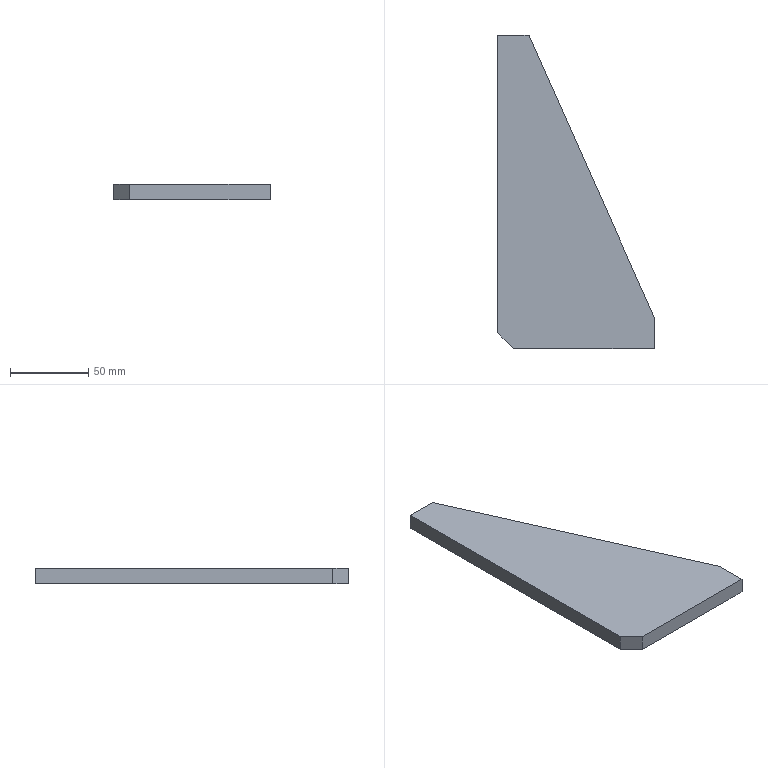Part | STEP file | Column base rib plate 1 | 1 solid | 8 faces | box 100 x 200 x 10 mm | volume 127500 mm3 | plane 8
STEP:
#1=CARTESIAN_POINT('',(0.,0.,0.));
#2=DIRECTION('',(0.,0.,1.));
#3=DIRECTION('',(1.,0.,0.));
#4=AXIS2_PLACEMENT_3D('',#1,#2,#3);
#5=CARTESIAN_POINT('',(0.,200.,-5.));
#6=VERTEX_POINT('',#5);
#7=CARTESIAN_POINT('',(0.,10.,-5.));
#8=VERTEX_POINT('',#7);
#9=CARTESIAN_POINT('',(0.,0.,-5.));
#10=DIRECTION('',(0.,-1.,0.));
#11=VECTOR('',#10,1.);
#12=LINE('',#9,#11);
#13=CARTESIAN_POINT('',(0.,0.,5.));
#14=DIRECTION('',(1.,0.,0.));
#15=DIRECTION('',(0.,0.,-1.));
#16=AXIS2_PLACEMENT_3D('',#13,#14,#15);
#17=PLANE('',#16);
#18=CARTESIAN_POINT('',(10.,0.));
#19=DIRECTION('',(0.,-1.));
#20=VECTOR('',#19,1.);
#21=LINE('',#18,#20);
#22=(GEOMETRIC_REPRESENTATION_CONTEXT(2)PARAMETRIC_REPRESENTATION_CONTEXT()REPRESENTATION_CONTEXT('',''));
#23=DEFINITIONAL_REPRESENTATION('',(#21),#22);
#24=PCURVE('',#17,#23);
#25=CARTESIAN_POINT('',(0.,0.,-5.));
#26=DIRECTION('',(0.,0.,-1.));
#27=DIRECTION('',(-1.,0.,0.));
#28=AXIS2_PLACEMENT_3D('',#25,#26,#27);
#29=PLANE('',#28);
#30=CARTESIAN_POINT('',(0.,0.));
#31=DIRECTION('',(0.,-1.));
#32=VECTOR('',#31,1.);
#33=LINE('',#30,#32);
#34=(GEOMETRIC_REPRESENTATION_CONTEXT(2)PARAMETRIC_REPRESENTATION_CONTEXT()REPRESENTATION_CONTEXT('',''));
#35=DEFINITIONAL_REPRESENTATION('',(#33),#34);
#36=PCURVE('',#29,#35);
#37=SURFACE_CURVE('',#12,(#24,#36),.PCURVE_S1.);
#38=EDGE_CURVE('',#6,#8,#37,.T.);
#39=ORIENTED_EDGE('',*,*,#38,.T.);
#40=CARTESIAN_POINT('',(0.,10.,5.));
#41=VERTEX_POINT('',#40);
#42=CARTESIAN_POINT('',(0.,10.,5.));
#43=DIRECTION('',(0.,0.,1.));
#44=VECTOR('',#43,1.);
#45=LINE('',#42,#44);
#46=CARTESIAN_POINT('',(0.,10.));
#47=DIRECTION('',(-1.,0.));
#48=VECTOR('',#47,1.);
#49=LINE('',#46,#48);
#50=(GEOMETRIC_REPRESENTATION_CONTEXT(2)PARAMETRIC_REPRESENTATION_CONTEXT()REPRESENTATION_CONTEXT('',''));
#51=DEFINITIONAL_REPRESENTATION('',(#49),#50);
#52=PCURVE('',#17,#51);
#53=CARTESIAN_POINT('',(10.,0.,5.));
#54=DIRECTION('',(0.7071,0.7071,0.));
#55=DIRECTION('',(0.,0.,-1.));
#56=AXIS2_PLACEMENT_3D('',#53,#54,#55);
#57=PLANE('',#56);
#58=CARTESIAN_POINT('',(0.,14.142));
#59=DIRECTION('',(-1.,0.));
#60=VECTOR('',#59,1.);
#61=LINE('',#58,#60);
#62=(GEOMETRIC_REPRESENTATION_CONTEXT(2)PARAMETRIC_REPRESENTATION_CONTEXT()REPRESENTATION_CONTEXT('',''));
#63=DEFINITIONAL_REPRESENTATION('',(#61),#62);
#64=PCURVE('',#57,#63);
#65=SURFACE_CURVE('',#45,(#52,#64),.PCURVE_S1.);
#66=EDGE_CURVE('',#8,#41,#65,.T.);
#67=ORIENTED_EDGE('',*,*,#66,.T.);
#68=CARTESIAN_POINT('',(0.,200.,5.));
#69=VERTEX_POINT('',#68);
#70=CARTESIAN_POINT('',(0.,0.,5.));
#71=DIRECTION('',(0.,-1.,0.));
#72=VECTOR('',#71,1.);
#73=LINE('',#70,#72);
#74=CARTESIAN_POINT('',(0.,0.));
#75=DIRECTION('',(0.,-1.));
#76=VECTOR('',#75,1.);
#77=LINE('',#74,#76);
#78=(GEOMETRIC_REPRESENTATION_CONTEXT(2)PARAMETRIC_REPRESENTATION_CONTEXT()REPRESENTATION_CONTEXT('',''));
#79=DEFINITIONAL_REPRESENTATION('',(#77),#78);
#80=PCURVE('',#17,#79);
#81=CARTESIAN_POINT('',(0.,0.,5.));
#82=DIRECTION('',(0.,0.,-1.));
#83=DIRECTION('',(-1.,0.,0.));
#84=AXIS2_PLACEMENT_3D('',#81,#82,#83);
#85=PLANE('',#84);
#86=CARTESIAN_POINT('',(0.,0.));
#87=DIRECTION('',(0.,-1.));
#88=VECTOR('',#87,1.);
#89=LINE('',#86,#88);
#90=(GEOMETRIC_REPRESENTATION_CONTEXT(2)PARAMETRIC_REPRESENTATION_CONTEXT()REPRESENTATION_CONTEXT('',''));
#91=DEFINITIONAL_REPRESENTATION('',(#89),#90);
#92=PCURVE('',#85,#91);
#93=SURFACE_CURVE('',#73,(#80,#92),.PCURVE_S1.);
#94=EDGE_CURVE('',#69,#41,#93,.T.);
#95=ORIENTED_EDGE('',*,*,#94,.F.);
#96=CARTESIAN_POINT('',(0.,200.,5.));
#97=DIRECTION('',(0.,0.,-1.));
#98=VECTOR('',#97,1.);
#99=LINE('',#96,#98);
#100=CARTESIAN_POINT('',(0.,200.));
#101=DIRECTION('',(1.,0.));
#102=VECTOR('',#101,1.);
#103=LINE('',#100,#102);
#104=(GEOMETRIC_REPRESENTATION_CONTEXT(2)PARAMETRIC_REPRESENTATION_CONTEXT()REPRESENTATION_CONTEXT('',''));
#105=DEFINITIONAL_REPRESENTATION('',(#103),#104);
#106=PCURVE('',#17,#105);
#107=CARTESIAN_POINT('',(0.,200.,5.));
#108=DIRECTION('',(0.,-1.,0.));
#109=DIRECTION('',(0.,0.,-1.));
#110=AXIS2_PLACEMENT_3D('',#107,#108,#109);
#111=PLANE('',#110);
#112=CARTESIAN_POINT('',(0.,0.));
#113=DIRECTION('',(1.,0.));
#114=VECTOR('',#113,1.);
#115=LINE('',#112,#114);
#116=(GEOMETRIC_REPRESENTATION_CONTEXT(2)PARAMETRIC_REPRESENTATION_CONTEXT()REPRESENTATION_CONTEXT('',''));
#117=DEFINITIONAL_REPRESENTATION('',(#115),#116);
#118=PCURVE('',#111,#117);
#119=SURFACE_CURVE('',#99,(#106,#118),.PCURVE_S1.);
#120=EDGE_CURVE('',#69,#6,#119,.T.);
#121=ORIENTED_EDGE('',*,*,#120,.T.);
#122=EDGE_LOOP('',(#39,#67,#95,#121));
#123=FACE_BOUND('',#122,.T.);
#124=ADVANCED_FACE('',(#123),#17,.F.);
#125=CARTESIAN_POINT('',(10.,0.,5.));
#126=VERTEX_POINT('',#125);
#127=CARTESIAN_POINT('',(100.,0.,5.));
#128=VERTEX_POINT('',#127);
#129=CARTESIAN_POINT('',(0.,0.,5.));
#130=DIRECTION('',(1.,0.,0.));
#131=VECTOR('',#130,1.);
#132=LINE('',#129,#131);
#133=CARTESIAN_POINT('',(0.,0.,5.));
#134=DIRECTION('',(0.,1.,0.));
#135=DIRECTION('',(0.,0.,1.));
#136=AXIS2_PLACEMENT_3D('',#133,#134,#135);
#137=PLANE('',#136);
#138=CARTESIAN_POINT('',(0.,0.));
#139=DIRECTION('',(0.,1.));
#140=VECTOR('',#139,1.);
#141=LINE('',#138,#140);
#142=(GEOMETRIC_REPRESENTATION_CONTEXT(2)PARAMETRIC_REPRESENTATION_CONTEXT()REPRESENTATION_CONTEXT('',''));
#143=DEFINITIONAL_REPRESENTATION('',(#141),#142);
#144=PCURVE('',#137,#143);
#145=CARTESIAN_POINT('',(0.,0.));
#146=DIRECTION('',(-1.,0.));
#147=VECTOR('',#146,1.);
#148=LINE('',#145,#147);
#149=(GEOMETRIC_REPRESENTATION_CONTEXT(2)PARAMETRIC_REPRESENTATION_CONTEXT()REPRESENTATION_CONTEXT('',''));
#150=DEFINITIONAL_REPRESENTATION('',(#148),#149);
#151=PCURVE('',#85,#150);
#152=SURFACE_CURVE('',#132,(#144,#151),.PCURVE_S1.);
#153=EDGE_CURVE('',#126,#128,#152,.T.);
#154=ORIENTED_EDGE('',*,*,#153,.F.);
#155=CARTESIAN_POINT('',(10.,0.,-5.));
#156=VERTEX_POINT('',#155);
#157=CARTESIAN_POINT('',(10.,0.,5.));
#158=DIRECTION('',(0.,0.,-1.));
#159=VECTOR('',#158,1.);
#160=LINE('',#157,#159);
#161=CARTESIAN_POINT('',(0.,10.));
#162=DIRECTION('',(-1.,0.));
#163=VECTOR('',#162,1.);
#164=LINE('',#161,#163);
#165=(GEOMETRIC_REPRESENTATION_CONTEXT(2)PARAMETRIC_REPRESENTATION_CONTEXT()REPRESENTATION_CONTEXT('',''));
#166=DEFINITIONAL_REPRESENTATION('',(#164),#165);
#167=PCURVE('',#137,#166);
#168=CARTESIAN_POINT('',(0.,0.));
#169=DIRECTION('',(1.,0.));
#170=VECTOR('',#169,1.);
#171=LINE('',#168,#170);
#172=(GEOMETRIC_REPRESENTATION_CONTEXT(2)PARAMETRIC_REPRESENTATION_CONTEXT()REPRESENTATION_CONTEXT('',''));
#173=DEFINITIONAL_REPRESENTATION('',(#171),#172);
#174=PCURVE('',#57,#173);
#175=SURFACE_CURVE('',#160,(#167,#174),.PCURVE_S1.);
#176=EDGE_CURVE('',#126,#156,#175,.T.);
#177=ORIENTED_EDGE('',*,*,#176,.T.);
#178=CARTESIAN_POINT('',(100.,0.,-5.));
#179=VERTEX_POINT('',#178);
#180=CARTESIAN_POINT('',(0.,0.,-5.));
#181=DIRECTION('',(1.,0.,0.));
#182=VECTOR('',#181,1.);
#183=LINE('',#180,#182);
#184=CARTESIAN_POINT('',(-10.,0.));
#185=DIRECTION('',(0.,1.));
#186=VECTOR('',#185,1.);
#187=LINE('',#184,#186);
#188=(GEOMETRIC_REPRESENTATION_CONTEXT(2)PARAMETRIC_REPRESENTATION_CONTEXT()REPRESENTATION_CONTEXT('',''));
#189=DEFINITIONAL_REPRESENTATION('',(#187),#188);
#190=PCURVE('',#137,#189);
#191=CARTESIAN_POINT('',(0.,0.));
#192=DIRECTION('',(-1.,0.));
#193=VECTOR('',#192,1.);
#194=LINE('',#191,#193);
#195=(GEOMETRIC_REPRESENTATION_CONTEXT(2)PARAMETRIC_REPRESENTATION_CONTEXT()REPRESENTATION_CONTEXT('',''));
#196=DEFINITIONAL_REPRESENTATION('',(#194),#195);
#197=PCURVE('',#29,#196);
#198=SURFACE_CURVE('',#183,(#190,#197),.PCURVE_S1.);
#199=EDGE_CURVE('',#156,#179,#198,.T.);
#200=ORIENTED_EDGE('',*,*,#199,.T.);
#201=CARTESIAN_POINT('',(100.,0.,5.));
#202=DIRECTION('',(0.,0.,-1.));
#203=VECTOR('',#202,1.);
#204=LINE('',#201,#203);
#205=CARTESIAN_POINT('',(0.,100.));
#206=DIRECTION('',(-1.,0.));
#207=VECTOR('',#206,1.);
#208=LINE('',#205,#207);
#209=(GEOMETRIC_REPRESENTATION_CONTEXT(2)PARAMETRIC_REPRESENTATION_CONTEXT()REPRESENTATION_CONTEXT('',''));
#210=DEFINITIONAL_REPRESENTATION('',(#208),#209);
#211=PCURVE('',#137,#210);
#212=CARTESIAN_POINT('',(100.,0.,5.));
#213=DIRECTION('',(-1.,0.,0.));
#214=DIRECTION('',(0.,-1.,0.));
#215=AXIS2_PLACEMENT_3D('',#212,#213,#214);
#216=PLANE('',#215);
#217=CARTESIAN_POINT('',(0.,0.));
#218=DIRECTION('',(0.,-1.));
#219=VECTOR('',#218,1.);
#220=LINE('',#217,#219);
#221=(GEOMETRIC_REPRESENTATION_CONTEXT(2)PARAMETRIC_REPRESENTATION_CONTEXT()REPRESENTATION_CONTEXT('',''));
#222=DEFINITIONAL_REPRESENTATION('',(#220),#221);
#223=PCURVE('',#216,#222);
#224=SURFACE_CURVE('',#204,(#211,#223),.PCURVE_S1.);
#225=EDGE_CURVE('',#128,#179,#224,.T.);
#226=ORIENTED_EDGE('',*,*,#225,.F.);
#227=EDGE_LOOP('',(#154,#177,#200,#226));
#228=FACE_BOUND('',#227,.T.);
#229=ADVANCED_FACE('',(#228),#137,.F.);
#230=CARTESIAN_POINT('',(100.,20.,-5.));
#231=VERTEX_POINT('',#230);
#232=CARTESIAN_POINT('',(100.,0.,-5.));
#233=DIRECTION('',(0.,1.,0.));
#234=VECTOR('',#233,1.);
#235=LINE('',#232,#234);
#236=CARTESIAN_POINT('',(0.,-10.));
#237=DIRECTION('',(-1.,0.));
#238=VECTOR('',#237,1.);
#239=LINE('',#236,#238);
#240=(GEOMETRIC_REPRESENTATION_CONTEXT(2)PARAMETRIC_REPRESENTATION_CONTEXT()REPRESENTATION_CONTEXT('',''));
#241=DEFINITIONAL_REPRESENTATION('',(#239),#240);
#242=PCURVE('',#216,#241);
#243=CARTESIAN_POINT('',(-100.,0.));
#244=DIRECTION('',(0.,1.));
#245=VECTOR('',#244,1.);
#246=LINE('',#243,#245);
#247=(GEOMETRIC_REPRESENTATION_CONTEXT(2)PARAMETRIC_REPRESENTATION_CONTEXT()REPRESENTATION_CONTEXT('',''));
#248=DEFINITIONAL_REPRESENTATION('',(#246),#247);
#249=PCURVE('',#29,#248);
#250=SURFACE_CURVE('',#235,(#242,#249),.PCURVE_S1.);
#251=EDGE_CURVE('',#179,#231,#250,.T.);
#252=ORIENTED_EDGE('',*,*,#251,.T.);
#253=CARTESIAN_POINT('',(100.,20.,5.));
#254=VERTEX_POINT('',#253);
#255=CARTESIAN_POINT('',(100.,20.,5.));
#256=DIRECTION('',(0.,0.,-1.));
#257=VECTOR('',#256,1.);
#258=LINE('',#255,#257);
#259=CARTESIAN_POINT('',(-20.,0.));
#260=DIRECTION('',(0.,-1.));
#261=VECTOR('',#260,1.);
#262=LINE('',#259,#261);
#263=(GEOMETRIC_REPRESENTATION_CONTEXT(2)PARAMETRIC_REPRESENTATION_CONTEXT()REPRESENTATION_CONTEXT('',''));
#264=DEFINITIONAL_REPRESENTATION('',(#262),#263);
#265=PCURVE('',#216,#264);
#266=CARTESIAN_POINT('',(100.,20.,5.));
#267=DIRECTION('',(-0.9138,-0.4061,0.));
#268=DIRECTION('',(0.4061,-0.9138,0.));
#269=AXIS2_PLACEMENT_3D('',#266,#267,#268);
#270=PLANE('',#269);
#271=CARTESIAN_POINT('',(0.,0.));
#272=DIRECTION('',(0.,-1.));
#273=VECTOR('',#272,1.);
#274=LINE('',#271,#273);
#275=(GEOMETRIC_REPRESENTATION_CONTEXT(2)PARAMETRIC_REPRESENTATION_CONTEXT()REPRESENTATION_CONTEXT('',''));
#276=DEFINITIONAL_REPRESENTATION('',(#274),#275);
#277=PCURVE('',#270,#276);
#278=SURFACE_CURVE('',#258,(#265,#277),.PCURVE_S1.);
#279=EDGE_CURVE('',#254,#231,#278,.T.);
#280=ORIENTED_EDGE('',*,*,#279,.F.);
#281=CARTESIAN_POINT('',(100.,0.,5.));
#282=DIRECTION('',(0.,1.,0.));
#283=VECTOR('',#282,1.);
#284=LINE('',#281,#283);
#285=CARTESIAN_POINT('',(0.,0.));
#286=DIRECTION('',(-1.,0.));
#287=VECTOR('',#286,1.);
#288=LINE('',#285,#287);
#289=(GEOMETRIC_REPRESENTATION_CONTEXT(2)PARAMETRIC_REPRESENTATION_CONTEXT()REPRESENTATION_CONTEXT('',''));
#290=DEFINITIONAL_REPRESENTATION('',(#288),#289);
#291=PCURVE('',#216,#290);
#292=CARTESIAN_POINT('',(-100.,0.));
#293=DIRECTION('',(0.,1.));
#294=VECTOR('',#293,1.);
#295=LINE('',#292,#294);
#296=(GEOMETRIC_REPRESENTATION_CONTEXT(2)PARAMETRIC_REPRESENTATION_CONTEXT()REPRESENTATION_CONTEXT('',''));
#297=DEFINITIONAL_REPRESENTATION('',(#295),#296);
#298=PCURVE('',#85,#297);
#299=SURFACE_CURVE('',#284,(#291,#298),.PCURVE_S1.);
#300=EDGE_CURVE('',#128,#254,#299,.T.);
#301=ORIENTED_EDGE('',*,*,#300,.F.);
#302=ORIENTED_EDGE('',*,*,#225,.T.);
#303=EDGE_LOOP('',(#252,#280,#301,#302));
#304=FACE_BOUND('',#303,.T.);
#305=ADVANCED_FACE('',(#304),#216,.F.);
#306=CARTESIAN_POINT('',(20.,200.,-5.));
#307=VERTEX_POINT('',#306);
#308=CARTESIAN_POINT('',(100.,20.,-5.));
#309=DIRECTION('',(-0.4061,0.9138,0.));
#310=VECTOR('',#309,1.);
#311=LINE('',#308,#310);
#312=CARTESIAN_POINT('',(0.,-10.));
#313=DIRECTION('',(-1.,0.));
#314=VECTOR('',#313,1.);
#315=LINE('',#312,#314);
#316=(GEOMETRIC_REPRESENTATION_CONTEXT(2)PARAMETRIC_REPRESENTATION_CONTEXT()REPRESENTATION_CONTEXT('',''));
#317=DEFINITIONAL_REPRESENTATION('',(#315),#316);
#318=PCURVE('',#270,#317);
#319=CARTESIAN_POINT('',(-100.,20.));
#320=DIRECTION('',(0.4061,0.9138));
#321=VECTOR('',#320,1.);
#322=LINE('',#319,#321);
#323=(GEOMETRIC_REPRESENTATION_CONTEXT(2)PARAMETRIC_REPRESENTATION_CONTEXT()REPRESENTATION_CONTEXT('',''));
#324=DEFINITIONAL_REPRESENTATION('',(#322),#323);
#325=PCURVE('',#29,#324);
#326=SURFACE_CURVE('',#311,(#318,#325),.PCURVE_S1.);
#327=EDGE_CURVE('',#231,#307,#326,.T.);
#328=ORIENTED_EDGE('',*,*,#327,.T.);
#329=CARTESIAN_POINT('',(20.,200.,5.));
#330=VERTEX_POINT('',#329);
#331=CARTESIAN_POINT('',(20.,200.,5.));
#332=DIRECTION('',(0.,0.,-1.));
#333=VECTOR('',#332,1.);
#334=LINE('',#331,#333);
#335=CARTESIAN_POINT('',(-196.977,0.));
#336=DIRECTION('',(0.,-1.));
#337=VECTOR('',#336,1.);
#338=LINE('',#335,#337);
#339=(GEOMETRIC_REPRESENTATION_CONTEXT(2)PARAMETRIC_REPRESENTATION_CONTEXT()REPRESENTATION_CONTEXT('',''));
#340=DEFINITIONAL_REPRESENTATION('',(#338),#339);
#341=PCURVE('',#270,#340);
#342=CARTESIAN_POINT('',(0.,20.));
#343=DIRECTION('',(1.,0.));
#344=VECTOR('',#343,1.);
#345=LINE('',#342,#344);
#346=(GEOMETRIC_REPRESENTATION_CONTEXT(2)PARAMETRIC_REPRESENTATION_CONTEXT()REPRESENTATION_CONTEXT('',''));
#347=DEFINITIONAL_REPRESENTATION('',(#345),#346);
#348=PCURVE('',#111,#347);
#349=SURFACE_CURVE('',#334,(#341,#348),.PCURVE_S1.);
#350=EDGE_CURVE('',#330,#307,#349,.T.);
#351=ORIENTED_EDGE('',*,*,#350,.F.);
#352=CARTESIAN_POINT('',(100.,20.,5.));
#353=DIRECTION('',(-0.4061,0.9138,0.));
#354=VECTOR('',#353,1.);
#355=LINE('',#352,#354);
#356=CARTESIAN_POINT('',(0.,0.));
#357=DIRECTION('',(-1.,0.));
#358=VECTOR('',#357,1.);
#359=LINE('',#356,#358);
#360=(GEOMETRIC_REPRESENTATION_CONTEXT(2)PARAMETRIC_REPRESENTATION_CONTEXT()REPRESENTATION_CONTEXT('',''));
#361=DEFINITIONAL_REPRESENTATION('',(#359),#360);
#362=PCURVE('',#270,#361);
#363=CARTESIAN_POINT('',(-100.,20.));
#364=DIRECTION('',(0.4061,0.9138));
#365=VECTOR('',#364,1.);
#366=LINE('',#363,#365);
#367=(GEOMETRIC_REPRESENTATION_CONTEXT(2)PARAMETRIC_REPRESENTATION_CONTEXT()REPRESENTATION_CONTEXT('',''));
#368=DEFINITIONAL_REPRESENTATION('',(#366),#367);
#369=PCURVE('',#85,#368);
#370=SURFACE_CURVE('',#355,(#362,#369),.PCURVE_S1.);
#371=EDGE_CURVE('',#254,#330,#370,.T.);
#372=ORIENTED_EDGE('',*,*,#371,.F.);
#373=ORIENTED_EDGE('',*,*,#279,.T.);
#374=EDGE_LOOP('',(#328,#351,#372,#373));
#375=FACE_BOUND('',#374,.T.);
#376=ADVANCED_FACE('',(#375),#270,.F.);
#377=CARTESIAN_POINT('',(0.,200.,-5.));
#378=DIRECTION('',(-1.,0.,0.));
#379=VECTOR('',#378,1.);
#380=LINE('',#377,#379);
#381=CARTESIAN_POINT('',(10.,0.));
#382=DIRECTION('',(0.,-1.));
#383=VECTOR('',#382,1.);
#384=LINE('',#381,#383);
#385=(GEOMETRIC_REPRESENTATION_CONTEXT(2)PARAMETRIC_REPRESENTATION_CONTEXT()REPRESENTATION_CONTEXT('',''));
#386=DEFINITIONAL_REPRESENTATION('',(#384),#385);
#387=PCURVE('',#111,#386);
#388=CARTESIAN_POINT('',(0.,200.));
#389=DIRECTION('',(1.,0.));
#390=VECTOR('',#389,1.);
#391=LINE('',#388,#390);
#392=(GEOMETRIC_REPRESENTATION_CONTEXT(2)PARAMETRIC_REPRESENTATION_CONTEXT()REPRESENTATION_CONTEXT('',''));
#393=DEFINITIONAL_REPRESENTATION('',(#391),#392);
#394=PCURVE('',#29,#393);
#395=SURFACE_CURVE('',#380,(#387,#394),.PCURVE_S1.);
#396=EDGE_CURVE('',#307,#6,#395,.T.);
#397=ORIENTED_EDGE('',*,*,#396,.T.);
#398=ORIENTED_EDGE('',*,*,#120,.F.);
#399=CARTESIAN_POINT('',(0.,200.,5.));
#400=DIRECTION('',(-1.,0.,0.));
#401=VECTOR('',#400,1.);
#402=LINE('',#399,#401);
#403=CARTESIAN_POINT('',(0.,0.));
#404=DIRECTION('',(0.,-1.));
#405=VECTOR('',#404,1.);
#406=LINE('',#403,#405);
#407=(GEOMETRIC_REPRESENTATION_CONTEXT(2)PARAMETRIC_REPRESENTATION_CONTEXT()REPRESENTATION_CONTEXT('',''));
#408=DEFINITIONAL_REPRESENTATION('',(#406),#407);
#409=PCURVE('',#111,#408);
#410=CARTESIAN_POINT('',(0.,200.));
#411=DIRECTION('',(1.,0.));
#412=VECTOR('',#411,1.);
#413=LINE('',#410,#412);
#414=(GEOMETRIC_REPRESENTATION_CONTEXT(2)PARAMETRIC_REPRESENTATION_CONTEXT()REPRESENTATION_CONTEXT('',''));
#415=DEFINITIONAL_REPRESENTATION('',(#413),#414);
#416=PCURVE('',#85,#415);
#417=SURFACE_CURVE('',#402,(#409,#416),.PCURVE_S1.);
#418=EDGE_CURVE('',#330,#69,#417,.T.);
#419=ORIENTED_EDGE('',*,*,#418,.F.);
#420=ORIENTED_EDGE('',*,*,#350,.T.);
#421=EDGE_LOOP('',(#397,#398,#419,#420));
#422=FACE_BOUND('',#421,.T.);
#423=ADVANCED_FACE('',(#422),#111,.F.);
#424=ORIENTED_EDGE('',*,*,#94,.T.);
#425=CARTESIAN_POINT('',(10.,0.,5.));
#426=DIRECTION('',(0.7071,-0.7071,0.));
#427=VECTOR('',#426,1.);
#428=LINE('',#425,#427);
#429=CARTESIAN_POINT('',(-10.,0.));
#430=DIRECTION('',(-0.7071,-0.7071));
#431=VECTOR('',#430,1.);
#432=LINE('',#429,#431);
#433=(GEOMETRIC_REPRESENTATION_CONTEXT(2)PARAMETRIC_REPRESENTATION_CONTEXT()REPRESENTATION_CONTEXT('',''));
#434=DEFINITIONAL_REPRESENTATION('',(#432),#433);
#435=PCURVE('',#85,#434);
#436=CARTESIAN_POINT('',(0.,0.));
#437=DIRECTION('',(0.,-1.));
#438=VECTOR('',#437,1.);
#439=LINE('',#436,#438);
#440=(GEOMETRIC_REPRESENTATION_CONTEXT(2)PARAMETRIC_REPRESENTATION_CONTEXT()REPRESENTATION_CONTEXT('',''));
#441=DEFINITIONAL_REPRESENTATION('',(#439),#440);
#442=PCURVE('',#57,#441);
#443=SURFACE_CURVE('',#428,(#435,#442),.PCURVE_S1.);
#444=EDGE_CURVE('',#41,#126,#443,.T.);
#445=ORIENTED_EDGE('',*,*,#444,.T.);
#446=ORIENTED_EDGE('',*,*,#153,.T.);
#447=ORIENTED_EDGE('',*,*,#300,.T.);
#448=ORIENTED_EDGE('',*,*,#371,.T.);
#449=ORIENTED_EDGE('',*,*,#418,.T.);
#450=EDGE_LOOP('',(#424,#445,#446,#447,#448,#449));
#451=FACE_BOUND('',#450,.T.);
#452=ADVANCED_FACE('',(#451),#85,.F.);
#453=ORIENTED_EDGE('',*,*,#199,.F.);
#454=CARTESIAN_POINT('',(5.,5.,-5.));
#455=DIRECTION('',(-0.7071,0.7071,0.));
#456=VECTOR('',#455,1.);
#457=LINE('',#454,#456);
#458=CARTESIAN_POINT('',(-5.,5.));
#459=DIRECTION('',(0.7071,0.7071));
#460=VECTOR('',#459,1.);
#461=LINE('',#458,#460);
#462=(GEOMETRIC_REPRESENTATION_CONTEXT(2)PARAMETRIC_REPRESENTATION_CONTEXT()REPRESENTATION_CONTEXT('',''));
#463=DEFINITIONAL_REPRESENTATION('',(#461),#462);
#464=PCURVE('',#29,#463);
#465=CARTESIAN_POINT('',(10.,7.071));
#466=DIRECTION('',(0.,1.));
#467=VECTOR('',#466,1.);
#468=LINE('',#465,#467);
#469=(GEOMETRIC_REPRESENTATION_CONTEXT(2)PARAMETRIC_REPRESENTATION_CONTEXT()REPRESENTATION_CONTEXT('',''));
#470=DEFINITIONAL_REPRESENTATION('',(#468),#469);
#471=PCURVE('',#57,#470);
#472=SURFACE_CURVE('',#457,(#464,#471),.PCURVE_S1.);
#473=EDGE_CURVE('',#156,#8,#472,.T.);
#474=ORIENTED_EDGE('',*,*,#473,.T.);
#475=ORIENTED_EDGE('',*,*,#38,.F.);
#476=ORIENTED_EDGE('',*,*,#396,.F.);
#477=ORIENTED_EDGE('',*,*,#327,.F.);
#478=ORIENTED_EDGE('',*,*,#251,.F.);
#479=EDGE_LOOP('',(#453,#474,#475,#476,#477,#478));
#480=FACE_BOUND('',#479,.T.);
#481=ADVANCED_FACE('',(#480),#29,.T.);
#482=ORIENTED_EDGE('',*,*,#444,.F.);
#483=ORIENTED_EDGE('',*,*,#66,.F.);
#484=ORIENTED_EDGE('',*,*,#473,.F.);
#485=ORIENTED_EDGE('',*,*,#176,.F.);
#486=EDGE_LOOP('',(#482,#483,#484,#485));
#487=FACE_BOUND('',#486,.T.);
#488=ADVANCED_FACE('',(#487),#57,.F.);
#489=CLOSED_SHELL('',(#124,#229,#305,#376,#423,#452,#481,#488));
#490=MANIFOLD_SOLID_BREP('',#489);
#491=(LENGTH_UNIT()NAMED_UNIT(*)SI_UNIT(.MILLI.,.METRE.));
#492=UNCERTAINTY_MEASURE_WITH_UNIT(LENGTH_MEASURE(0.0000001),#491,'','');
#493=(NAMED_UNIT(*)PLANE_ANGLE_UNIT()SI_UNIT($,.RADIAN.));
#494=(NAMED_UNIT(*)SI_UNIT($,.STERADIAN.)SOLID_ANGLE_UNIT());
#495=(GEOMETRIC_REPRESENTATION_CONTEXT(3)GLOBAL_UNCERTAINTY_ASSIGNED_CONTEXT((#492))GLOBAL_UNIT_ASSIGNED_CONTEXT((#491,#493,#494))REPRESENTATION_CONTEXT('',''));
#496=ADVANCED_BREP_SHAPE_REPRESENTATION('',(#4,#490),#495);